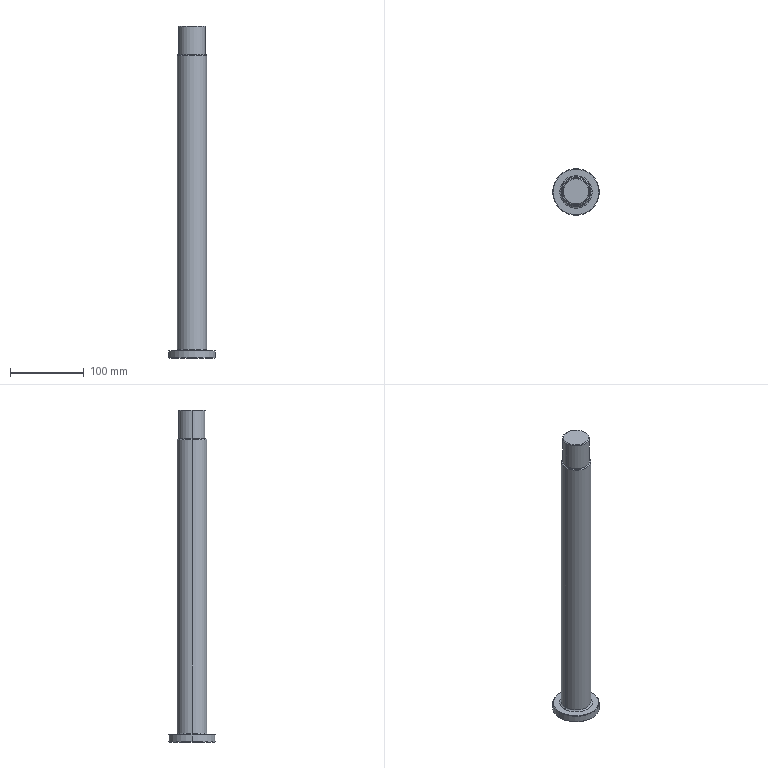Part | SolidWorks | features Chamfer 2, ICE 2, Extrusion 1, Fillet 1 | 1 solid | 20 faces | box 63 x 63 x 449 mm | volume 573468 mm3 | cone 8 | cylinder 6 | plane 4 | torus 2 | commonest cylinder face diameters 36 x2 40 x2 63 x2
STEP:
#1=CARTESIAN_POINT('',(-31.,0.,0.));
#2=VERTEX_POINT('',#1);
#3=CARTESIAN_POINT('',(31.,0.,0.));
#4=VERTEX_POINT('',#3);
#5=CARTESIAN_POINT('',(0.,0.,0.));
#6=DIRECTION('',(0.,0.,-1.));
#7=DIRECTION('',(1.,0.,0.));
#8=AXIS2_PLACEMENT_3D('',#5,#6,#7);
#9=CIRCLE('',#8,31.);
#10=EDGE_CURVE('',#2,#4,#9,.T.);
#11=ORIENTED_EDGE('',*,*,#10,.F.);
#12=CARTESIAN_POINT('',(-31.5,0.,0.5));
#13=VERTEX_POINT('',#12);
#14=CARTESIAN_POINT('',(-31.5,0.,0.5));
#15=DIRECTION('',(-0.7071,0.,0.7071));
#16=VECTOR('',#15,1000.);
#17=LINE('',#14,#16);
#18=EDGE_CURVE('',#2,#13,#17,.T.);
#19=ORIENTED_EDGE('',*,*,#18,.T.);
#20=CARTESIAN_POINT('',(31.5,0.,0.5));
#21=VERTEX_POINT('',#20);
#22=CARTESIAN_POINT('',(0.,0.,0.5));
#23=DIRECTION('',(0.,0.,1.));
#24=DIRECTION('',(1.,0.,0.));
#25=AXIS2_PLACEMENT_3D('',#22,#23,#24);
#26=CIRCLE('',#25,31.5);
#27=EDGE_CURVE('',#21,#13,#26,.T.);
#28=ORIENTED_EDGE('',*,*,#27,.F.);
#29=CARTESIAN_POINT('',(31.5,0.,0.5));
#30=DIRECTION('',(0.7071,0.,0.7071));
#31=VECTOR('',#30,1000.);
#32=LINE('',#29,#31);
#33=EDGE_CURVE('',#4,#21,#32,.T.);
#34=ORIENTED_EDGE('',*,*,#33,.F.);
#35=EDGE_LOOP('',(#11,#19,#28,#34));
#36=FACE_OUTER_BOUND('',#35,.T.);
#37=CARTESIAN_POINT('',(0.,0.,0.5));
#38=DIRECTION('',(0.,0.,1.));
#39=DIRECTION('',(1.,0.,0.));
#40=AXIS2_PLACEMENT_3D('',#37,#38,#39);
#41=CONICAL_SURFACE('',#40,31.5,0.7854);
#42=ADVANCED_FACE('',(#36),#41,.T.);
#43=CARTESIAN_POINT('',(31.,0.,10.));
#44=VERTEX_POINT('',#43);
#45=CARTESIAN_POINT('',(-31.,0.,10.));
#46=VERTEX_POINT('',#45);
#47=CARTESIAN_POINT('',(0.,0.,10.));
#48=DIRECTION('',(0.,0.,1.));
#49=DIRECTION('',(1.,0.,0.));
#50=AXIS2_PLACEMENT_3D('',#47,#48,#49);
#51=CIRCLE('',#50,31.);
#52=EDGE_CURVE('',#44,#46,#51,.T.);
#53=ORIENTED_EDGE('',*,*,#52,.F.);
#54=CARTESIAN_POINT('',(31.5,0.,9.5));
#55=VERTEX_POINT('',#54);
#56=CARTESIAN_POINT('',(31.,0.,10.));
#57=DIRECTION('',(0.7071,0.,-0.7071));
#58=VECTOR('',#57,1000.);
#59=LINE('',#56,#58);
#60=EDGE_CURVE('',#44,#55,#59,.T.);
#61=ORIENTED_EDGE('',*,*,#60,.T.);
#62=CARTESIAN_POINT('',(-31.5,0.,9.5));
#63=VERTEX_POINT('',#62);
#64=CARTESIAN_POINT('',(0.,0.,9.5));
#65=DIRECTION('',(0.,0.,-1.));
#66=DIRECTION('',(1.,0.,0.));
#67=AXIS2_PLACEMENT_3D('',#64,#65,#66);
#68=CIRCLE('',#67,31.5);
#69=EDGE_CURVE('',#63,#55,#68,.T.);
#70=ORIENTED_EDGE('',*,*,#69,.F.);
#71=CARTESIAN_POINT('',(-31.,0.,10.));
#72=DIRECTION('',(-0.7071,0.,-0.7071));
#73=VECTOR('',#72,1000.);
#74=LINE('',#71,#73);
#75=EDGE_CURVE('',#46,#63,#74,.T.);
#76=ORIENTED_EDGE('',*,*,#75,.F.);
#77=EDGE_LOOP('',(#53,#61,#70,#76));
#78=FACE_OUTER_BOUND('',#77,.T.);
#79=CARTESIAN_POINT('',(0.,0.,10.));
#80=DIRECTION('',(0.,0.,-1.));
#81=DIRECTION('',(-1.,0.,0.));
#82=AXIS2_PLACEMENT_3D('',#79,#80,#81);
#83=CONICAL_SURFACE('',#82,31.,0.7854);
#84=ADVANCED_FACE('',(#78),#83,.T.);
#85=CARTESIAN_POINT('',(19.,0.,410.));
#86=VERTEX_POINT('',#85);
#87=CARTESIAN_POINT('',(-19.,0.,410.));
#88=VERTEX_POINT('',#87);
#89=CARTESIAN_POINT('',(0.,0.,410.));
#90=DIRECTION('',(0.,0.,1.));
#91=DIRECTION('',(1.,0.,0.));
#92=AXIS2_PLACEMENT_3D('',#89,#90,#91);
#93=CIRCLE('',#92,19.);
#94=EDGE_CURVE('',#86,#88,#93,.T.);
#95=ORIENTED_EDGE('',*,*,#94,.F.);
#96=CARTESIAN_POINT('',(20.,0.,409.));
#97=VERTEX_POINT('',#96);
#98=CARTESIAN_POINT('',(19.,0.,410.));
#99=DIRECTION('',(0.7071,0.,-0.7071));
#100=VECTOR('',#99,1000.);
#101=LINE('',#98,#100);
#102=EDGE_CURVE('',#86,#97,#101,.T.);
#103=ORIENTED_EDGE('',*,*,#102,.T.);
#104=CARTESIAN_POINT('',(-20.,0.,409.));
#105=VERTEX_POINT('',#104);
#106=CARTESIAN_POINT('',(0.,0.,409.));
#107=DIRECTION('',(0.,0.,-1.));
#108=DIRECTION('',(1.,0.,0.));
#109=AXIS2_PLACEMENT_3D('',#106,#107,#108);
#110=CIRCLE('',#109,20.);
#111=EDGE_CURVE('',#105,#97,#110,.T.);
#112=ORIENTED_EDGE('',*,*,#111,.F.);
#113=CARTESIAN_POINT('',(-19.,0.,410.));
#114=DIRECTION('',(-0.7071,0.,-0.7071));
#115=VECTOR('',#114,1000.);
#116=LINE('',#113,#115);
#117=EDGE_CURVE('',#88,#105,#116,.T.);
#118=ORIENTED_EDGE('',*,*,#117,.F.);
#119=EDGE_LOOP('',(#95,#103,#112,#118));
#120=FACE_OUTER_BOUND('',#119,.T.);
#121=CARTESIAN_POINT('',(0.,0.,410.));
#122=DIRECTION('',(0.,0.,-1.));
#123=DIRECTION('',(-1.,0.,0.));
#124=AXIS2_PLACEMENT_3D('',#121,#122,#123);
#125=CONICAL_SURFACE('',#124,19.,0.7854);
#126=ADVANCED_FACE('',(#120),#125,.T.);
#127=CARTESIAN_POINT('',(17.,0.,449.));
#128=VERTEX_POINT('',#127);
#129=CARTESIAN_POINT('',(-17.,0.,449.));
#130=VERTEX_POINT('',#129);
#131=CARTESIAN_POINT('',(0.,0.,449.));
#132=DIRECTION('',(0.,0.,1.));
#133=DIRECTION('',(1.,0.,0.));
#134=AXIS2_PLACEMENT_3D('',#131,#132,#133);
#135=CIRCLE('',#134,17.);
#136=EDGE_CURVE('',#128,#130,#135,.T.);
#137=ORIENTED_EDGE('',*,*,#136,.F.);
#138=CARTESIAN_POINT('',(18.,0.,448.));
#139=VERTEX_POINT('',#138);
#140=CARTESIAN_POINT('',(17.,0.,449.));
#141=DIRECTION('',(0.7071,0.,-0.7071));
#142=VECTOR('',#141,1000.);
#143=LINE('',#140,#142);
#144=EDGE_CURVE('',#128,#139,#143,.T.);
#145=ORIENTED_EDGE('',*,*,#144,.T.);
#146=CARTESIAN_POINT('',(-18.,0.,448.));
#147=VERTEX_POINT('',#146);
#148=CARTESIAN_POINT('',(0.,0.,448.));
#149=DIRECTION('',(0.,0.,-1.));
#150=DIRECTION('',(1.,0.,0.));
#151=AXIS2_PLACEMENT_3D('',#148,#149,#150);
#152=CIRCLE('',#151,18.);
#153=EDGE_CURVE('',#147,#139,#152,.T.);
#154=ORIENTED_EDGE('',*,*,#153,.F.);
#155=CARTESIAN_POINT('',(-17.,0.,449.));
#156=DIRECTION('',(-0.7071,0.,-0.7071));
#157=VECTOR('',#156,1000.);
#158=LINE('',#155,#157);
#159=EDGE_CURVE('',#130,#147,#158,.T.);
#160=ORIENTED_EDGE('',*,*,#159,.F.);
#161=EDGE_LOOP('',(#137,#145,#154,#160));
#162=FACE_OUTER_BOUND('',#161,.T.);
#163=CARTESIAN_POINT('',(0.,0.,449.));
#164=DIRECTION('',(0.,0.,-1.));
#165=DIRECTION('',(-1.,0.,0.));
#166=AXIS2_PLACEMENT_3D('',#163,#164,#165);
#167=CONICAL_SURFACE('',#166,17.,0.7854);
#168=ADVANCED_FACE('',(#162),#167,.T.);
#169=CARTESIAN_POINT('',(-20.,0.,12.));
#170=VERTEX_POINT('',#169);
#171=CARTESIAN_POINT('',(20.,0.,12.));
#172=VERTEX_POINT('',#171);
#173=CARTESIAN_POINT('',(0.,0.,12.));
#174=DIRECTION('',(0.,0.,1.));
#175=DIRECTION('',(1.,0.,0.));
#176=AXIS2_PLACEMENT_3D('',#173,#174,#175);
#177=CIRCLE('',#176,20.);
#178=EDGE_CURVE('',#170,#172,#177,.T.);
#179=ORIENTED_EDGE('',*,*,#178,.F.);
#180=CARTESIAN_POINT('',(-22.,0.,10.));
#181=VERTEX_POINT('',#180);
#182=CARTESIAN_POINT('',(-22.,0.,12.));
#183=DIRECTION('',(0.,1.,0.));
#184=DIRECTION('',(-1.,0.,0.));
#185=AXIS2_PLACEMENT_3D('',#182,#183,#184);
#186=CIRCLE('',#185,2.);
#187=EDGE_CURVE('',#170,#181,#186,.T.);
#188=ORIENTED_EDGE('',*,*,#187,.T.);
#189=CARTESIAN_POINT('',(22.,0.,10.));
#190=VERTEX_POINT('',#189);
#191=CARTESIAN_POINT('',(0.,0.,10.));
#192=DIRECTION('',(0.,0.,-1.));
#193=DIRECTION('',(1.,0.,0.));
#194=AXIS2_PLACEMENT_3D('',#191,#192,#193);
#195=CIRCLE('',#194,22.);
#196=EDGE_CURVE('',#190,#181,#195,.T.);
#197=ORIENTED_EDGE('',*,*,#196,.F.);
#198=CARTESIAN_POINT('',(22.,0.,12.));
#199=DIRECTION('',(0.,-1.,0.));
#200=DIRECTION('',(0.,0.,-1.));
#201=AXIS2_PLACEMENT_3D('',#198,#199,#200);
#202=CIRCLE('',#201,2.);
#203=EDGE_CURVE('',#172,#190,#202,.T.);
#204=ORIENTED_EDGE('',*,*,#203,.F.);
#205=EDGE_LOOP('',(#179,#188,#197,#204));
#206=FACE_OUTER_BOUND('',#205,.T.);
#207=CARTESIAN_POINT('',(0.,0.,12.));
#208=DIRECTION('',(0.,0.,1.));
#209=DIRECTION('',(1.,0.,0.));
#210=AXIS2_PLACEMENT_3D('',#207,#208,#209);
#211=TOROIDAL_SURFACE('',#210,22.,2.);
#212=ADVANCED_FACE('',(#206),#211,.F.);
#213=ORIENTED_EDGE('',*,*,#153,.T.);
#214=CARTESIAN_POINT('',(18.,0.,410.));
#215=VERTEX_POINT('',#214);
#216=CARTESIAN_POINT('',(18.,0.,449.));
#217=DIRECTION('',(0.,0.,-1.));
#218=VECTOR('',#217,1000.);
#219=LINE('',#216,#218);
#220=EDGE_CURVE('',#139,#215,#219,.T.);
#221=ORIENTED_EDGE('',*,*,#220,.T.);
#222=CARTESIAN_POINT('',(-18.,0.,410.));
#223=VERTEX_POINT('',#222);
#224=CARTESIAN_POINT('',(0.,0.,410.));
#225=DIRECTION('',(0.,0.,1.));
#226=DIRECTION('',(1.,0.,0.));
#227=AXIS2_PLACEMENT_3D('',#224,#225,#226);
#228=CIRCLE('',#227,18.);
#229=EDGE_CURVE('',#215,#223,#228,.T.);
#230=ORIENTED_EDGE('',*,*,#229,.T.);
#231=CARTESIAN_POINT('',(-18.,0.,449.));
#232=DIRECTION('',(0.,0.,-1.));
#233=VECTOR('',#232,1000.);
#234=LINE('',#231,#233);
#235=EDGE_CURVE('',#147,#223,#234,.T.);
#236=ORIENTED_EDGE('',*,*,#235,.F.);
#237=EDGE_LOOP('',(#213,#221,#230,#236));
#238=FACE_OUTER_BOUND('',#237,.T.);
#239=CARTESIAN_POINT('',(0.,0.,449.));
#240=DIRECTION('',(0.,0.,-1.));
#241=DIRECTION('',(-1.,0.,0.));
#242=AXIS2_PLACEMENT_3D('',#239,#240,#241);
#243=CYLINDRICAL_SURFACE('',#242,18.);
#244=ADVANCED_FACE('',(#238),#243,.T.);
#245=ORIENTED_EDGE('',*,*,#111,.T.);
#246=CARTESIAN_POINT('',(20.,0.,410.));
#247=DIRECTION('',(0.,0.,-1.));
#248=VECTOR('',#247,1000.);
#249=LINE('',#246,#248);
#250=EDGE_CURVE('',#97,#172,#249,.T.);
#251=ORIENTED_EDGE('',*,*,#250,.T.);
#252=CARTESIAN_POINT('',(0.,0.,12.));
#253=DIRECTION('',(0.,0.,1.));
#254=DIRECTION('',(1.,0.,0.));
#255=AXIS2_PLACEMENT_3D('',#252,#253,#254);
#256=CIRCLE('',#255,20.);
#257=EDGE_CURVE('',#172,#170,#256,.T.);
#258=ORIENTED_EDGE('',*,*,#257,.T.);
#259=CARTESIAN_POINT('',(-20.,0.,410.));
#260=DIRECTION('',(0.,0.,-1.));
#261=VECTOR('',#260,1000.);
#262=LINE('',#259,#261);
#263=EDGE_CURVE('',#105,#170,#262,.T.);
#264=ORIENTED_EDGE('',*,*,#263,.F.);
#265=EDGE_LOOP('',(#245,#251,#258,#264));
#266=FACE_OUTER_BOUND('',#265,.T.);
#267=CARTESIAN_POINT('',(0.,0.,410.));
#268=DIRECTION('',(0.,0.,-1.));
#269=DIRECTION('',(-1.,0.,0.));
#270=AXIS2_PLACEMENT_3D('',#267,#268,#269);
#271=CYLINDRICAL_SURFACE('',#270,20.);
#272=ADVANCED_FACE('',(#266),#271,.T.);
#273=ORIENTED_EDGE('',*,*,#69,.T.);
#274=CARTESIAN_POINT('',(31.5,0.,10.));
#275=DIRECTION('',(0.,0.,-1.));
#276=VECTOR('',#275,1000.);
#277=LINE('',#274,#276);
#278=EDGE_CURVE('',#55,#21,#277,.T.);
#279=ORIENTED_EDGE('',*,*,#278,.T.);
#280=ORIENTED_EDGE('',*,*,#27,.T.);
#281=CARTESIAN_POINT('',(-31.5,0.,10.));
#282=DIRECTION('',(0.,0.,-1.));
#283=VECTOR('',#282,1000.);
#284=LINE('',#281,#283);
#285=EDGE_CURVE('',#63,#13,#284,.T.);
#286=ORIENTED_EDGE('',*,*,#285,.F.);
#287=EDGE_LOOP('',(#273,#279,#280,#286));
#288=FACE_OUTER_BOUND('',#287,.T.);
#289=CARTESIAN_POINT('',(0.,0.,10.));
#290=DIRECTION('',(0.,0.,-1.));
#291=DIRECTION('',(-1.,0.,0.));
#292=AXIS2_PLACEMENT_3D('',#289,#290,#291);
#293=CYLINDRICAL_SURFACE('',#292,31.5);
#294=ADVANCED_FACE('',(#288),#293,.T.);
#295=CARTESIAN_POINT('',(0.,0.,410.));
#296=DIRECTION('',(0.,0.,1.));
#297=DIRECTION('',(1.,0.,0.));
#298=AXIS2_PLACEMENT_3D('',#295,#296,#297);
#299=CIRCLE('',#298,19.);
#300=EDGE_CURVE('',#88,#86,#299,.T.);
#301=ORIENTED_EDGE('',*,*,#300,.T.);
#302=ORIENTED_EDGE('',*,*,#94,.T.);
#303=EDGE_LOOP('',(#301,#302));
#304=FACE_OUTER_BOUND('',#303,.T.);
#305=CARTESIAN_POINT('',(0.,0.,410.));
#306=DIRECTION('',(0.,0.,1.));
#307=DIRECTION('',(1.,0.,0.));
#308=AXIS2_PLACEMENT_3D('',#305,#306,#307);
#309=CIRCLE('',#308,18.);
#310=EDGE_CURVE('',#223,#215,#309,.T.);
#311=ORIENTED_EDGE('',*,*,#310,.F.);
#312=ORIENTED_EDGE('',*,*,#229,.F.);
#313=EDGE_LOOP('',(#311,#312));
#314=FACE_BOUND('',#313,.T.);
#315=CARTESIAN_POINT('',(0.,0.,410.));
#316=DIRECTION('',(0.,0.,1.));
#317=DIRECTION('',(1.,0.,0.));
#318=AXIS2_PLACEMENT_3D('',#315,#316,#317);
#319=PLANE('',#318);
#320=ADVANCED_FACE('',(#304,#314),#319,.T.);
#321=CARTESIAN_POINT('',(0.,0.,10.));
#322=DIRECTION('',(0.,0.,1.));
#323=DIRECTION('',(1.,0.,0.));
#324=AXIS2_PLACEMENT_3D('',#321,#322,#323);
#325=CIRCLE('',#324,31.);
#326=EDGE_CURVE('',#46,#44,#325,.T.);
#327=ORIENTED_EDGE('',*,*,#326,.T.);
#328=ORIENTED_EDGE('',*,*,#52,.T.);
#329=EDGE_LOOP('',(#327,#328));
#330=FACE_OUTER_BOUND('',#329,.T.);
#331=ORIENTED_EDGE('',*,*,#196,.T.);
#332=CARTESIAN_POINT('',(0.,0.,10.));
#333=DIRECTION('',(0.,0.,-1.));
#334=DIRECTION('',(1.,0.,0.));
#335=AXIS2_PLACEMENT_3D('',#332,#333,#334);
#336=CIRCLE('',#335,22.);
#337=EDGE_CURVE('',#181,#190,#336,.T.);
#338=ORIENTED_EDGE('',*,*,#337,.T.);
#339=EDGE_LOOP('',(#331,#338));
#340=FACE_BOUND('',#339,.T.);
#341=CARTESIAN_POINT('',(0.,0.,10.));
#342=DIRECTION('',(0.,0.,1.));
#343=DIRECTION('',(1.,0.,0.));
#344=AXIS2_PLACEMENT_3D('',#341,#342,#343);
#345=PLANE('',#344);
#346=ADVANCED_FACE('',(#330,#340),#345,.T.);
#347=ORIENTED_EDGE('',*,*,#278,.F.);
#348=CARTESIAN_POINT('',(0.,0.,9.5));
#349=DIRECTION('',(0.,0.,-1.));
#350=DIRECTION('',(1.,0.,0.));
#351=AXIS2_PLACEMENT_3D('',#348,#349,#350);
#352=CIRCLE('',#351,31.5);
#353=EDGE_CURVE('',#55,#63,#352,.T.);
#354=ORIENTED_EDGE('',*,*,#353,.T.);
#355=ORIENTED_EDGE('',*,*,#285,.T.);
#356=CARTESIAN_POINT('',(0.,0.,0.5));
#357=DIRECTION('',(0.,0.,1.));
#358=DIRECTION('',(1.,0.,0.));
#359=AXIS2_PLACEMENT_3D('',#356,#357,#358);
#360=CIRCLE('',#359,31.5);
#361=EDGE_CURVE('',#13,#21,#360,.T.);
#362=ORIENTED_EDGE('',*,*,#361,.T.);
#363=EDGE_LOOP('',(#347,#354,#355,#362));
#364=FACE_OUTER_BOUND('',#363,.T.);
#365=CARTESIAN_POINT('',(0.,0.,10.));
#366=DIRECTION('',(0.,0.,-1.));
#367=DIRECTION('',(-1.,0.,0.));
#368=AXIS2_PLACEMENT_3D('',#365,#366,#367);
#369=CYLINDRICAL_SURFACE('',#368,31.5);
#370=ADVANCED_FACE('',(#364),#369,.T.);
#371=CARTESIAN_POINT('',(0.,0.,0.));
#372=DIRECTION('',(0.,0.,-1.));
#373=DIRECTION('',(1.,0.,0.));
#374=AXIS2_PLACEMENT_3D('',#371,#372,#373);
#375=CIRCLE('',#374,31.);
#376=EDGE_CURVE('',#4,#2,#375,.T.);
#377=ORIENTED_EDGE('',*,*,#376,.T.);
#378=ORIENTED_EDGE('',*,*,#10,.T.);
#379=EDGE_LOOP('',(#377,#378));
#380=FACE_OUTER_BOUND('',#379,.T.);
#381=CARTESIAN_POINT('',(0.,0.,0.));
#382=DIRECTION('',(0.,0.,1.));
#383=DIRECTION('',(1.,0.,0.));
#384=AXIS2_PLACEMENT_3D('',#381,#382,#383);
#385=PLANE('',#384);
#386=ADVANCED_FACE('',(#380),#385,.F.);
#387=ORIENTED_EDGE('',*,*,#250,.F.);
#388=CARTESIAN_POINT('',(0.,0.,409.));
#389=DIRECTION('',(0.,0.,-1.));
#390=DIRECTION('',(1.,0.,0.));
#391=AXIS2_PLACEMENT_3D('',#388,#389,#390);
#392=CIRCLE('',#391,20.);
#393=EDGE_CURVE('',#97,#105,#392,.T.);
#394=ORIENTED_EDGE('',*,*,#393,.T.);
#395=ORIENTED_EDGE('',*,*,#263,.T.);
#396=ORIENTED_EDGE('',*,*,#178,.T.);
#397=EDGE_LOOP('',(#387,#394,#395,#396));
#398=FACE_OUTER_BOUND('',#397,.T.);
#399=CARTESIAN_POINT('',(0.,0.,410.));
#400=DIRECTION('',(0.,0.,-1.));
#401=DIRECTION('',(-1.,0.,0.));
#402=AXIS2_PLACEMENT_3D('',#399,#400,#401);
#403=CYLINDRICAL_SURFACE('',#402,20.);
#404=ADVANCED_FACE('',(#398),#403,.T.);
#405=ORIENTED_EDGE('',*,*,#220,.F.);
#406=CARTESIAN_POINT('',(0.,0.,448.));
#407=DIRECTION('',(0.,0.,-1.));
#408=DIRECTION('',(1.,0.,0.));
#409=AXIS2_PLACEMENT_3D('',#406,#407,#408);
#410=CIRCLE('',#409,18.);
#411=EDGE_CURVE('',#139,#147,#410,.T.);
#412=ORIENTED_EDGE('',*,*,#411,.T.);
#413=ORIENTED_EDGE('',*,*,#235,.T.);
#414=ORIENTED_EDGE('',*,*,#310,.T.);
#415=EDGE_LOOP('',(#405,#412,#413,#414));
#416=FACE_OUTER_BOUND('',#415,.T.);
#417=CARTESIAN_POINT('',(0.,0.,449.));
#418=DIRECTION('',(0.,0.,-1.));
#419=DIRECTION('',(-1.,0.,0.));
#420=AXIS2_PLACEMENT_3D('',#417,#418,#419);
#421=CYLINDRICAL_SURFACE('',#420,18.);
#422=ADVANCED_FACE('',(#416),#421,.T.);
#423=CARTESIAN_POINT('',(0.,0.,449.));
#424=DIRECTION('',(0.,0.,1.));
#425=DIRECTION('',(1.,0.,0.));
#426=AXIS2_PLACEMENT_3D('',#423,#424,#425);
#427=CIRCLE('',#426,17.);
#428=EDGE_CURVE('',#130,#128,#427,.T.);
#429=ORIENTED_EDGE('',*,*,#428,.T.);
#430=ORIENTED_EDGE('',*,*,#136,.T.);
#431=EDGE_LOOP('',(#429,#430));
#432=FACE_OUTER_BOUND('',#431,.T.);
#433=CARTESIAN_POINT('',(0.,0.,449.));
#434=DIRECTION('',(0.,0.,1.));
#435=DIRECTION('',(1.,0.,0.));
#436=AXIS2_PLACEMENT_3D('',#433,#434,#435);
#437=PLANE('',#436);
#438=ADVANCED_FACE('',(#432),#437,.T.);
#439=ORIENTED_EDGE('',*,*,#187,.F.);
#440=ORIENTED_EDGE('',*,*,#257,.F.);
#441=ORIENTED_EDGE('',*,*,#203,.T.);
#442=ORIENTED_EDGE('',*,*,#337,.F.);
#443=EDGE_LOOP('',(#439,#440,#441,#442));
#444=FACE_OUTER_BOUND('',#443,.T.);
#445=CARTESIAN_POINT('',(0.,0.,12.));
#446=DIRECTION('',(0.,0.,1.));
#447=DIRECTION('',(1.,0.,0.));
#448=AXIS2_PLACEMENT_3D('',#445,#446,#447);
#449=TOROIDAL_SURFACE('',#448,22.,2.);
#450=ADVANCED_FACE('',(#444),#449,.F.);
#451=ORIENTED_EDGE('',*,*,#144,.F.);
#452=ORIENTED_EDGE('',*,*,#428,.F.);
#453=ORIENTED_EDGE('',*,*,#159,.T.);
#454=ORIENTED_EDGE('',*,*,#411,.F.);
#455=EDGE_LOOP('',(#451,#452,#453,#454));
#456=FACE_OUTER_BOUND('',#455,.T.);
#457=CARTESIAN_POINT('',(0.,0.,449.));
#458=DIRECTION('',(0.,0.,-1.));
#459=DIRECTION('',(-1.,0.,0.));
#460=AXIS2_PLACEMENT_3D('',#457,#458,#459);
#461=CONICAL_SURFACE('',#460,17.,0.7854);
#462=ADVANCED_FACE('',(#456),#461,.T.);
#463=ORIENTED_EDGE('',*,*,#102,.F.);
#464=ORIENTED_EDGE('',*,*,#300,.F.);
#465=ORIENTED_EDGE('',*,*,#117,.T.);
#466=ORIENTED_EDGE('',*,*,#393,.F.);
#467=EDGE_LOOP('',(#463,#464,#465,#466));
#468=FACE_OUTER_BOUND('',#467,.T.);
#469=CARTESIAN_POINT('',(0.,0.,410.));
#470=DIRECTION('',(0.,0.,-1.));
#471=DIRECTION('',(-1.,0.,0.));
#472=AXIS2_PLACEMENT_3D('',#469,#470,#471);
#473=CONICAL_SURFACE('',#472,19.,0.7854);
#474=ADVANCED_FACE('',(#468),#473,.T.);
#475=ORIENTED_EDGE('',*,*,#60,.F.);
#476=ORIENTED_EDGE('',*,*,#326,.F.);
#477=ORIENTED_EDGE('',*,*,#75,.T.);
#478=ORIENTED_EDGE('',*,*,#353,.F.);
#479=EDGE_LOOP('',(#475,#476,#477,#478));
#480=FACE_OUTER_BOUND('',#479,.T.);
#481=CARTESIAN_POINT('',(0.,0.,10.));
#482=DIRECTION('',(0.,0.,-1.));
#483=DIRECTION('',(-1.,0.,0.));
#484=AXIS2_PLACEMENT_3D('',#481,#482,#483);
#485=CONICAL_SURFACE('',#484,31.,0.7854);
#486=ADVANCED_FACE('',(#480),#485,.T.);
#487=ORIENTED_EDGE('',*,*,#18,.F.);
#488=ORIENTED_EDGE('',*,*,#376,.F.);
#489=ORIENTED_EDGE('',*,*,#33,.T.);
#490=ORIENTED_EDGE('',*,*,#361,.F.);
#491=EDGE_LOOP('',(#487,#488,#489,#490));
#492=FACE_OUTER_BOUND('',#491,.T.);
#493=CARTESIAN_POINT('',(0.,0.,0.5));
#494=DIRECTION('',(0.,0.,1.));
#495=DIRECTION('',(1.,0.,0.));
#496=AXIS2_PLACEMENT_3D('',#493,#494,#495);
#497=CONICAL_SURFACE('',#496,31.5,0.7854);
#498=ADVANCED_FACE('',(#492),#497,.T.);
#499=CLOSED_SHELL('',(#42,#84,#126,#168,#212,#244,#272,#294,#320,#346,#370,#386,#404,#422,#438,#450,#462,#474,#486,#498));
#500=MANIFOLD_SOLID_BREP('',#499);
#501=CARTESIAN_POINT('',(0.,0.,0.));
#502=DIRECTION('',(0.,0.,1.));
#503=DIRECTION('',(1.,0.,0.));
#504=AXIS2_PLACEMENT_3D('',#501,#502,#503);
#505=(LENGTH_UNIT()NAMED_UNIT(*)SI_UNIT(.MILLI.,.METRE.));
#506=UNCERTAINTY_MEASURE_WITH_UNIT(LENGTH_MEASURE(0.00001),#505,'','');
#507=(NAMED_UNIT(*)PLANE_ANGLE_UNIT()SI_UNIT($,.RADIAN.));
#508=(NAMED_UNIT(*)SI_UNIT($,.STERADIAN.)SOLID_ANGLE_UNIT());
#509=(GEOMETRIC_REPRESENTATION_CONTEXT(3)GLOBAL_UNCERTAINTY_ASSIGNED_CONTEXT((#506))GLOBAL_UNIT_ASSIGNED_CONTEXT((#505,#507,#508))REPRESENTATION_CONTEXT('',''));
#510=ADVANCED_BREP_SHAPE_REPRESENTATION('',(#500,#504),#509);